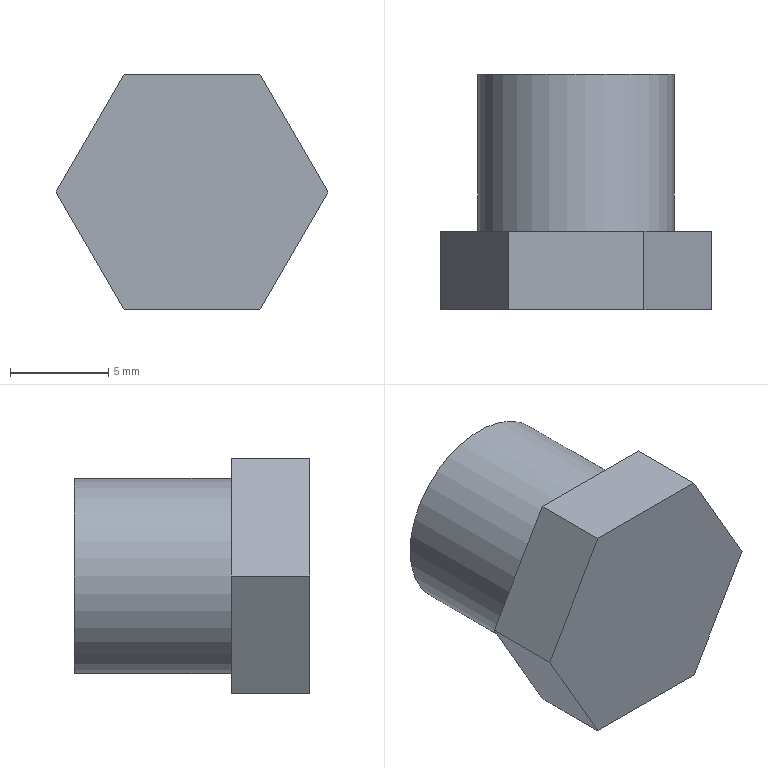Part | STEP file | 1-06.3 | 1 solid | 10 faces | box 13.856 x 12 x 12 mm | volume 1127 mm3 | plane 9 | cylinder 1 | commonest cylinder face diameters 10 x1
STEP:
#1=CARTESIAN_POINT('',(0.,0.,0.));
#2=DIRECTION('',(0.,0.,1.));
#3=DIRECTION('',(1.,0.,0.));
#4=AXIS2_PLACEMENT_3D('',#1,#2,#3);
#5=CARTESIAN_POINT('',(-6.928,-4.,0.));
#6=VERTEX_POINT('',#5);
#7=CARTESIAN_POINT('',(-3.464,-4.,6.));
#8=VERTEX_POINT('',#7);
#9=CARTESIAN_POINT('',(-6.928,-4.,0.));
#10=DIRECTION('',(0.5,0.,0.866));
#11=VECTOR('',#10,1.);
#12=LINE('',#9,#11);
#13=CARTESIAN_POINT('',(0.,-4.,-0.9282));
#14=DIRECTION('',(0.,1.,0.));
#15=DIRECTION('',(1.,0.,0.));
#16=AXIS2_PLACEMENT_3D('',#13,#14,#15);
#17=PLANE('',#16);
#18=CARTESIAN_POINT('',(-6.928,-0.9282));
#19=DIRECTION('',(0.5,-0.866));
#20=VECTOR('',#19,1.);
#21=LINE('',#18,#20);
#22=(GEOMETRIC_REPRESENTATION_CONTEXT(2)PARAMETRIC_REPRESENTATION_CONTEXT()REPRESENTATION_CONTEXT('',''));
#23=DEFINITIONAL_REPRESENTATION('',(#21),#22);
#24=PCURVE('',#17,#23);
#25=CARTESIAN_POINT('',(-5.196,-2.,3.));
#26=DIRECTION('',(0.866,0.,-0.5));
#27=DIRECTION('',(0.5,0.,0.866));
#28=AXIS2_PLACEMENT_3D('',#25,#26,#27);
#29=PLANE('',#28);
#30=CARTESIAN_POINT('',(-3.464,2.));
#31=DIRECTION('',(1.,0.));
#32=VECTOR('',#31,1.);
#33=LINE('',#30,#32);
#34=(GEOMETRIC_REPRESENTATION_CONTEXT(2)PARAMETRIC_REPRESENTATION_CONTEXT()REPRESENTATION_CONTEXT('',''));
#35=DEFINITIONAL_REPRESENTATION('',(#33),#34);
#36=PCURVE('',#29,#35);
#37=SURFACE_CURVE('',#12,(#24,#36),.PCURVE_S1.);
#38=EDGE_CURVE('',#6,#8,#37,.T.);
#39=ORIENTED_EDGE('',*,*,#38,.T.);
#40=CARTESIAN_POINT('',(3.464,-4.,6.));
#41=VERTEX_POINT('',#40);
#42=CARTESIAN_POINT('',(-3.464,-4.,6.));
#43=DIRECTION('',(1.,0.,0.));
#44=VECTOR('',#43,1.);
#45=LINE('',#42,#44);
#46=CARTESIAN_POINT('',(-3.464,-6.928));
#47=DIRECTION('',(1.,0.));
#48=VECTOR('',#47,1.);
#49=LINE('',#46,#48);
#50=(GEOMETRIC_REPRESENTATION_CONTEXT(2)PARAMETRIC_REPRESENTATION_CONTEXT()REPRESENTATION_CONTEXT('',''));
#51=DEFINITIONAL_REPRESENTATION('',(#49),#50);
#52=PCURVE('',#17,#51);
#53=CARTESIAN_POINT('',(0.,-2.,6.));
#54=DIRECTION('',(0.,0.,-1.));
#55=DIRECTION('',(1.,0.,0.));
#56=AXIS2_PLACEMENT_3D('',#53,#54,#55);
#57=PLANE('',#56);
#58=CARTESIAN_POINT('',(-3.464,2.));
#59=DIRECTION('',(1.,0.));
#60=VECTOR('',#59,1.);
#61=LINE('',#58,#60);
#62=(GEOMETRIC_REPRESENTATION_CONTEXT(2)PARAMETRIC_REPRESENTATION_CONTEXT()REPRESENTATION_CONTEXT('',''));
#63=DEFINITIONAL_REPRESENTATION('',(#61),#62);
#64=PCURVE('',#57,#63);
#65=SURFACE_CURVE('',#45,(#52,#64),.PCURVE_S1.);
#66=EDGE_CURVE('',#8,#41,#65,.T.);
#67=ORIENTED_EDGE('',*,*,#66,.T.);
#68=CARTESIAN_POINT('',(6.928,-4.,0.));
#69=VERTEX_POINT('',#68);
#70=CARTESIAN_POINT('',(3.464,-4.,6.));
#71=DIRECTION('',(0.5,0.,-0.866));
#72=VECTOR('',#71,1.);
#73=LINE('',#70,#72);
#74=CARTESIAN_POINT('',(3.464,-6.928));
#75=DIRECTION('',(0.5,0.866));
#76=VECTOR('',#75,1.);
#77=LINE('',#74,#76);
#78=(GEOMETRIC_REPRESENTATION_CONTEXT(2)PARAMETRIC_REPRESENTATION_CONTEXT()REPRESENTATION_CONTEXT('',''));
#79=DEFINITIONAL_REPRESENTATION('',(#77),#78);
#80=PCURVE('',#17,#79);
#81=CARTESIAN_POINT('',(5.196,-2.,3.));
#82=DIRECTION('',(-0.866,0.,-0.5));
#83=DIRECTION('',(0.5,0.,-0.866));
#84=AXIS2_PLACEMENT_3D('',#81,#82,#83);
#85=PLANE('',#84);
#86=CARTESIAN_POINT('',(-3.464,2.));
#87=DIRECTION('',(1.,0.));
#88=VECTOR('',#87,1.);
#89=LINE('',#86,#88);
#90=(GEOMETRIC_REPRESENTATION_CONTEXT(2)PARAMETRIC_REPRESENTATION_CONTEXT()REPRESENTATION_CONTEXT('',''));
#91=DEFINITIONAL_REPRESENTATION('',(#89),#90);
#92=PCURVE('',#85,#91);
#93=SURFACE_CURVE('',#73,(#80,#92),.PCURVE_S1.);
#94=EDGE_CURVE('',#41,#69,#93,.T.);
#95=ORIENTED_EDGE('',*,*,#94,.T.);
#96=CARTESIAN_POINT('',(3.464,-4.,-6.));
#97=VERTEX_POINT('',#96);
#98=CARTESIAN_POINT('',(6.928,-4.,0.));
#99=DIRECTION('',(-0.5,0.,-0.866));
#100=VECTOR('',#99,1.);
#101=LINE('',#98,#100);
#102=CARTESIAN_POINT('',(6.928,-0.9282));
#103=DIRECTION('',(-0.5,0.866));
#104=VECTOR('',#103,1.);
#105=LINE('',#102,#104);
#106=(GEOMETRIC_REPRESENTATION_CONTEXT(2)PARAMETRIC_REPRESENTATION_CONTEXT()REPRESENTATION_CONTEXT('',''));
#107=DEFINITIONAL_REPRESENTATION('',(#105),#106);
#108=PCURVE('',#17,#107);
#109=CARTESIAN_POINT('',(5.196,-2.,-3.));
#110=DIRECTION('',(-0.866,0.,0.5));
#111=DIRECTION('',(-0.5,0.,-0.866));
#112=AXIS2_PLACEMENT_3D('',#109,#110,#111);
#113=PLANE('',#112);
#114=CARTESIAN_POINT('',(-3.464,2.));
#115=DIRECTION('',(1.,0.));
#116=VECTOR('',#115,1.);
#117=LINE('',#114,#116);
#118=(GEOMETRIC_REPRESENTATION_CONTEXT(2)PARAMETRIC_REPRESENTATION_CONTEXT()REPRESENTATION_CONTEXT('',''));
#119=DEFINITIONAL_REPRESENTATION('',(#117),#118);
#120=PCURVE('',#113,#119);
#121=SURFACE_CURVE('',#101,(#108,#120),.PCURVE_S1.);
#122=EDGE_CURVE('',#69,#97,#121,.T.);
#123=ORIENTED_EDGE('',*,*,#122,.T.);
#124=CARTESIAN_POINT('',(-3.464,-4.,-6.));
#125=VERTEX_POINT('',#124);
#126=CARTESIAN_POINT('',(3.464,-4.,-6.));
#127=DIRECTION('',(-1.,0.,0.));
#128=VECTOR('',#127,1.);
#129=LINE('',#126,#128);
#130=CARTESIAN_POINT('',(3.464,5.072));
#131=DIRECTION('',(-1.,0.));
#132=VECTOR('',#131,1.);
#133=LINE('',#130,#132);
#134=(GEOMETRIC_REPRESENTATION_CONTEXT(2)PARAMETRIC_REPRESENTATION_CONTEXT()REPRESENTATION_CONTEXT('',''));
#135=DEFINITIONAL_REPRESENTATION('',(#133),#134);
#136=PCURVE('',#17,#135);
#137=CARTESIAN_POINT('',(0.,-2.,-6.));
#138=DIRECTION('',(0.,0.,1.));
#139=DIRECTION('',(-1.,0.,0.));
#140=AXIS2_PLACEMENT_3D('',#137,#138,#139);
#141=PLANE('',#140);
#142=CARTESIAN_POINT('',(-3.464,2.));
#143=DIRECTION('',(1.,0.));
#144=VECTOR('',#143,1.);
#145=LINE('',#142,#144);
#146=(GEOMETRIC_REPRESENTATION_CONTEXT(2)PARAMETRIC_REPRESENTATION_CONTEXT()REPRESENTATION_CONTEXT('',''));
#147=DEFINITIONAL_REPRESENTATION('',(#145),#146);
#148=PCURVE('',#141,#147);
#149=SURFACE_CURVE('',#129,(#136,#148),.PCURVE_S1.);
#150=EDGE_CURVE('',#97,#125,#149,.T.);
#151=ORIENTED_EDGE('',*,*,#150,.T.);
#152=CARTESIAN_POINT('',(-3.464,-4.,-6.));
#153=DIRECTION('',(-0.5,0.,0.866));
#154=VECTOR('',#153,1.);
#155=LINE('',#152,#154);
#156=CARTESIAN_POINT('',(-3.464,5.072));
#157=DIRECTION('',(-0.5,-0.866));
#158=VECTOR('',#157,1.);
#159=LINE('',#156,#158);
#160=(GEOMETRIC_REPRESENTATION_CONTEXT(2)PARAMETRIC_REPRESENTATION_CONTEXT()REPRESENTATION_CONTEXT('',''));
#161=DEFINITIONAL_REPRESENTATION('',(#159),#160);
#162=PCURVE('',#17,#161);
#163=CARTESIAN_POINT('',(-5.196,-2.,-3.));
#164=DIRECTION('',(0.866,0.,0.5));
#165=DIRECTION('',(-0.5,0.,0.866));
#166=AXIS2_PLACEMENT_3D('',#163,#164,#165);
#167=PLANE('',#166);
#168=CARTESIAN_POINT('',(-3.464,2.));
#169=DIRECTION('',(1.,0.));
#170=VECTOR('',#169,1.);
#171=LINE('',#168,#170);
#172=(GEOMETRIC_REPRESENTATION_CONTEXT(2)PARAMETRIC_REPRESENTATION_CONTEXT()REPRESENTATION_CONTEXT('',''));
#173=DEFINITIONAL_REPRESENTATION('',(#171),#172);
#174=PCURVE('',#167,#173);
#175=SURFACE_CURVE('',#155,(#162,#174),.PCURVE_S1.);
#176=EDGE_CURVE('',#125,#6,#175,.T.);
#177=ORIENTED_EDGE('',*,*,#176,.T.);
#178=EDGE_LOOP('',(#39,#67,#95,#123,#151,#177));
#179=FACE_BOUND('',#178,.F.);
#180=ADVANCED_FACE('',(#179),#17,.F.);
#181=CARTESIAN_POINT('',(-6.928,0.,0.));
#182=VERTEX_POINT('',#181);
#183=CARTESIAN_POINT('',(-3.464,0.,6.));
#184=VERTEX_POINT('',#183);
#185=CARTESIAN_POINT('',(-6.928,0.,0.));
#186=DIRECTION('',(0.5,0.,0.866));
#187=VECTOR('',#186,1.);
#188=LINE('',#185,#187);
#189=CARTESIAN_POINT('',(-3.464,-2.));
#190=DIRECTION('',(1.,0.));
#191=VECTOR('',#190,1.);
#192=LINE('',#189,#191);
#193=(GEOMETRIC_REPRESENTATION_CONTEXT(2)PARAMETRIC_REPRESENTATION_CONTEXT()REPRESENTATION_CONTEXT('',''));
#194=DEFINITIONAL_REPRESENTATION('',(#192),#193);
#195=PCURVE('',#29,#194);
#196=CARTESIAN_POINT('',(0.,0.,-0.9282));
#197=DIRECTION('',(0.,1.,0.));
#198=DIRECTION('',(1.,0.,0.));
#199=AXIS2_PLACEMENT_3D('',#196,#197,#198);
#200=PLANE('',#199);
#201=CARTESIAN_POINT('',(-6.928,-0.9282));
#202=DIRECTION('',(0.5,-0.866));
#203=VECTOR('',#202,1.);
#204=LINE('',#201,#203);
#205=(GEOMETRIC_REPRESENTATION_CONTEXT(2)PARAMETRIC_REPRESENTATION_CONTEXT()REPRESENTATION_CONTEXT('',''));
#206=DEFINITIONAL_REPRESENTATION('',(#204),#205);
#207=PCURVE('',#200,#206);
#208=SURFACE_CURVE('',#188,(#195,#207),.PCURVE_S1.);
#209=EDGE_CURVE('',#182,#184,#208,.T.);
#210=ORIENTED_EDGE('',*,*,#209,.T.);
#211=CARTESIAN_POINT('',(-3.464,0.,6.));
#212=DIRECTION('',(0.,-1.,0.));
#213=VECTOR('',#212,1.);
#214=LINE('',#211,#213);
#215=CARTESIAN_POINT('',(3.464,-2.));
#216=DIRECTION('',(0.,1.));
#217=VECTOR('',#216,1.);
#218=LINE('',#215,#217);
#219=(GEOMETRIC_REPRESENTATION_CONTEXT(2)PARAMETRIC_REPRESENTATION_CONTEXT()REPRESENTATION_CONTEXT('',''));
#220=DEFINITIONAL_REPRESENTATION('',(#218),#219);
#221=PCURVE('',#29,#220);
#222=CARTESIAN_POINT('',(-3.464,-2.));
#223=DIRECTION('',(0.,1.));
#224=VECTOR('',#223,1.);
#225=LINE('',#222,#224);
#226=(GEOMETRIC_REPRESENTATION_CONTEXT(2)PARAMETRIC_REPRESENTATION_CONTEXT()REPRESENTATION_CONTEXT('',''));
#227=DEFINITIONAL_REPRESENTATION('',(#225),#226);
#228=PCURVE('',#57,#227);
#229=SURFACE_CURVE('',#214,(#221,#228),.PCURVE_S1.);
#230=EDGE_CURVE('',#184,#8,#229,.T.);
#231=ORIENTED_EDGE('',*,*,#230,.T.);
#232=ORIENTED_EDGE('',*,*,#38,.F.);
#233=CARTESIAN_POINT('',(-6.928,0.,0.));
#234=DIRECTION('',(0.,-1.,0.));
#235=VECTOR('',#234,1.);
#236=LINE('',#233,#235);
#237=CARTESIAN_POINT('',(-3.464,-2.));
#238=DIRECTION('',(0.,1.));
#239=VECTOR('',#238,1.);
#240=LINE('',#237,#239);
#241=(GEOMETRIC_REPRESENTATION_CONTEXT(2)PARAMETRIC_REPRESENTATION_CONTEXT()REPRESENTATION_CONTEXT('',''));
#242=DEFINITIONAL_REPRESENTATION('',(#240),#241);
#243=PCURVE('',#29,#242);
#244=CARTESIAN_POINT('',(3.464,-2.));
#245=DIRECTION('',(0.,1.));
#246=VECTOR('',#245,1.);
#247=LINE('',#244,#246);
#248=(GEOMETRIC_REPRESENTATION_CONTEXT(2)PARAMETRIC_REPRESENTATION_CONTEXT()REPRESENTATION_CONTEXT('',''));
#249=DEFINITIONAL_REPRESENTATION('',(#247),#248);
#250=PCURVE('',#167,#249);
#251=SURFACE_CURVE('',#236,(#243,#250),.PCURVE_S1.);
#252=EDGE_CURVE('',#182,#6,#251,.T.);
#253=ORIENTED_EDGE('',*,*,#252,.F.);
#254=EDGE_LOOP('',(#210,#231,#232,#253));
#255=FACE_BOUND('',#254,.F.);
#256=ADVANCED_FACE('',(#255),#29,.F.);
#257=CARTESIAN_POINT('',(3.464,0.,6.));
#258=VERTEX_POINT('',#257);
#259=CARTESIAN_POINT('',(-3.464,0.,6.));
#260=DIRECTION('',(1.,0.,0.));
#261=VECTOR('',#260,1.);
#262=LINE('',#259,#261);
#263=CARTESIAN_POINT('',(-3.464,-2.));
#264=DIRECTION('',(1.,0.));
#265=VECTOR('',#264,1.);
#266=LINE('',#263,#265);
#267=(GEOMETRIC_REPRESENTATION_CONTEXT(2)PARAMETRIC_REPRESENTATION_CONTEXT()REPRESENTATION_CONTEXT('',''));
#268=DEFINITIONAL_REPRESENTATION('',(#266),#267);
#269=PCURVE('',#57,#268);
#270=CARTESIAN_POINT('',(-3.464,-6.928));
#271=DIRECTION('',(1.,0.));
#272=VECTOR('',#271,1.);
#273=LINE('',#270,#272);
#274=(GEOMETRIC_REPRESENTATION_CONTEXT(2)PARAMETRIC_REPRESENTATION_CONTEXT()REPRESENTATION_CONTEXT('',''));
#275=DEFINITIONAL_REPRESENTATION('',(#273),#274);
#276=PCURVE('',#200,#275);
#277=SURFACE_CURVE('',#262,(#269,#276),.PCURVE_S1.);
#278=EDGE_CURVE('',#184,#258,#277,.T.);
#279=ORIENTED_EDGE('',*,*,#278,.T.);
#280=CARTESIAN_POINT('',(3.464,0.,6.));
#281=DIRECTION('',(0.,-1.,0.));
#282=VECTOR('',#281,1.);
#283=LINE('',#280,#282);
#284=CARTESIAN_POINT('',(3.464,-2.));
#285=DIRECTION('',(0.,1.));
#286=VECTOR('',#285,1.);
#287=LINE('',#284,#286);
#288=(GEOMETRIC_REPRESENTATION_CONTEXT(2)PARAMETRIC_REPRESENTATION_CONTEXT()REPRESENTATION_CONTEXT('',''));
#289=DEFINITIONAL_REPRESENTATION('',(#287),#288);
#290=PCURVE('',#57,#289);
#291=CARTESIAN_POINT('',(-3.464,-2.));
#292=DIRECTION('',(0.,1.));
#293=VECTOR('',#292,1.);
#294=LINE('',#291,#293);
#295=(GEOMETRIC_REPRESENTATION_CONTEXT(2)PARAMETRIC_REPRESENTATION_CONTEXT()REPRESENTATION_CONTEXT('',''));
#296=DEFINITIONAL_REPRESENTATION('',(#294),#295);
#297=PCURVE('',#85,#296);
#298=SURFACE_CURVE('',#283,(#290,#297),.PCURVE_S1.);
#299=EDGE_CURVE('',#258,#41,#298,.T.);
#300=ORIENTED_EDGE('',*,*,#299,.T.);
#301=ORIENTED_EDGE('',*,*,#66,.F.);
#302=ORIENTED_EDGE('',*,*,#230,.F.);
#303=EDGE_LOOP('',(#279,#300,#301,#302));
#304=FACE_BOUND('',#303,.F.);
#305=ADVANCED_FACE('',(#304),#57,.F.);
#306=CARTESIAN_POINT('',(6.928,0.,0.));
#307=VERTEX_POINT('',#306);
#308=CARTESIAN_POINT('',(3.464,0.,6.));
#309=DIRECTION('',(0.5,0.,-0.866));
#310=VECTOR('',#309,1.);
#311=LINE('',#308,#310);
#312=CARTESIAN_POINT('',(-3.464,-2.));
#313=DIRECTION('',(1.,0.));
#314=VECTOR('',#313,1.);
#315=LINE('',#312,#314);
#316=(GEOMETRIC_REPRESENTATION_CONTEXT(2)PARAMETRIC_REPRESENTATION_CONTEXT()REPRESENTATION_CONTEXT('',''));
#317=DEFINITIONAL_REPRESENTATION('',(#315),#316);
#318=PCURVE('',#85,#317);
#319=CARTESIAN_POINT('',(3.464,-6.928));
#320=DIRECTION('',(0.5,0.866));
#321=VECTOR('',#320,1.);
#322=LINE('',#319,#321);
#323=(GEOMETRIC_REPRESENTATION_CONTEXT(2)PARAMETRIC_REPRESENTATION_CONTEXT()REPRESENTATION_CONTEXT('',''));
#324=DEFINITIONAL_REPRESENTATION('',(#322),#323);
#325=PCURVE('',#200,#324);
#326=SURFACE_CURVE('',#311,(#318,#325),.PCURVE_S1.);
#327=EDGE_CURVE('',#258,#307,#326,.T.);
#328=ORIENTED_EDGE('',*,*,#327,.T.);
#329=CARTESIAN_POINT('',(6.928,0.,0.));
#330=DIRECTION('',(0.,-1.,0.));
#331=VECTOR('',#330,1.);
#332=LINE('',#329,#331);
#333=CARTESIAN_POINT('',(3.464,-2.));
#334=DIRECTION('',(0.,1.));
#335=VECTOR('',#334,1.);
#336=LINE('',#333,#335);
#337=(GEOMETRIC_REPRESENTATION_CONTEXT(2)PARAMETRIC_REPRESENTATION_CONTEXT()REPRESENTATION_CONTEXT('',''));
#338=DEFINITIONAL_REPRESENTATION('',(#336),#337);
#339=PCURVE('',#85,#338);
#340=CARTESIAN_POINT('',(-3.464,-2.));
#341=DIRECTION('',(0.,1.));
#342=VECTOR('',#341,1.);
#343=LINE('',#340,#342);
#344=(GEOMETRIC_REPRESENTATION_CONTEXT(2)PARAMETRIC_REPRESENTATION_CONTEXT()REPRESENTATION_CONTEXT('',''));
#345=DEFINITIONAL_REPRESENTATION('',(#343),#344);
#346=PCURVE('',#113,#345);
#347=SURFACE_CURVE('',#332,(#339,#346),.PCURVE_S1.);
#348=EDGE_CURVE('',#307,#69,#347,.T.);
#349=ORIENTED_EDGE('',*,*,#348,.T.);
#350=ORIENTED_EDGE('',*,*,#94,.F.);
#351=ORIENTED_EDGE('',*,*,#299,.F.);
#352=EDGE_LOOP('',(#328,#349,#350,#351));
#353=FACE_BOUND('',#352,.F.);
#354=ADVANCED_FACE('',(#353),#85,.F.);
#355=CARTESIAN_POINT('',(3.464,0.,-6.));
#356=VERTEX_POINT('',#355);
#357=CARTESIAN_POINT('',(6.928,0.,0.));
#358=DIRECTION('',(-0.5,0.,-0.866));
#359=VECTOR('',#358,1.);
#360=LINE('',#357,#359);
#361=CARTESIAN_POINT('',(-3.464,-2.));
#362=DIRECTION('',(1.,0.));
#363=VECTOR('',#362,1.);
#364=LINE('',#361,#363);
#365=(GEOMETRIC_REPRESENTATION_CONTEXT(2)PARAMETRIC_REPRESENTATION_CONTEXT()REPRESENTATION_CONTEXT('',''));
#366=DEFINITIONAL_REPRESENTATION('',(#364),#365);
#367=PCURVE('',#113,#366);
#368=CARTESIAN_POINT('',(6.928,-0.9282));
#369=DIRECTION('',(-0.5,0.866));
#370=VECTOR('',#369,1.);
#371=LINE('',#368,#370);
#372=(GEOMETRIC_REPRESENTATION_CONTEXT(2)PARAMETRIC_REPRESENTATION_CONTEXT()REPRESENTATION_CONTEXT('',''));
#373=DEFINITIONAL_REPRESENTATION('',(#371),#372);
#374=PCURVE('',#200,#373);
#375=SURFACE_CURVE('',#360,(#367,#374),.PCURVE_S1.);
#376=EDGE_CURVE('',#307,#356,#375,.T.);
#377=ORIENTED_EDGE('',*,*,#376,.T.);
#378=CARTESIAN_POINT('',(3.464,0.,-6.));
#379=DIRECTION('',(0.,-1.,0.));
#380=VECTOR('',#379,1.);
#381=LINE('',#378,#380);
#382=CARTESIAN_POINT('',(3.464,-2.));
#383=DIRECTION('',(0.,1.));
#384=VECTOR('',#383,1.);
#385=LINE('',#382,#384);
#386=(GEOMETRIC_REPRESENTATION_CONTEXT(2)PARAMETRIC_REPRESENTATION_CONTEXT()REPRESENTATION_CONTEXT('',''));
#387=DEFINITIONAL_REPRESENTATION('',(#385),#386);
#388=PCURVE('',#113,#387);
#389=CARTESIAN_POINT('',(-3.464,-2.));
#390=DIRECTION('',(0.,1.));
#391=VECTOR('',#390,1.);
#392=LINE('',#389,#391);
#393=(GEOMETRIC_REPRESENTATION_CONTEXT(2)PARAMETRIC_REPRESENTATION_CONTEXT()REPRESENTATION_CONTEXT('',''));
#394=DEFINITIONAL_REPRESENTATION('',(#392),#393);
#395=PCURVE('',#141,#394);
#396=SURFACE_CURVE('',#381,(#388,#395),.PCURVE_S1.);
#397=EDGE_CURVE('',#356,#97,#396,.T.);
#398=ORIENTED_EDGE('',*,*,#397,.T.);
#399=ORIENTED_EDGE('',*,*,#122,.F.);
#400=ORIENTED_EDGE('',*,*,#348,.F.);
#401=EDGE_LOOP('',(#377,#398,#399,#400));
#402=FACE_BOUND('',#401,.F.);
#403=ADVANCED_FACE('',(#402),#113,.F.);
#404=CARTESIAN_POINT('',(-3.464,0.,-6.));
#405=VERTEX_POINT('',#404);
#406=CARTESIAN_POINT('',(3.464,0.,-6.));
#407=DIRECTION('',(-1.,0.,0.));
#408=VECTOR('',#407,1.);
#409=LINE('',#406,#408);
#410=CARTESIAN_POINT('',(-3.464,-2.));
#411=DIRECTION('',(1.,0.));
#412=VECTOR('',#411,1.);
#413=LINE('',#410,#412);
#414=(GEOMETRIC_REPRESENTATION_CONTEXT(2)PARAMETRIC_REPRESENTATION_CONTEXT()REPRESENTATION_CONTEXT('',''));
#415=DEFINITIONAL_REPRESENTATION('',(#413),#414);
#416=PCURVE('',#141,#415);
#417=CARTESIAN_POINT('',(3.464,5.072));
#418=DIRECTION('',(-1.,0.));
#419=VECTOR('',#418,1.);
#420=LINE('',#417,#419);
#421=(GEOMETRIC_REPRESENTATION_CONTEXT(2)PARAMETRIC_REPRESENTATION_CONTEXT()REPRESENTATION_CONTEXT('',''));
#422=DEFINITIONAL_REPRESENTATION('',(#420),#421);
#423=PCURVE('',#200,#422);
#424=SURFACE_CURVE('',#409,(#416,#423),.PCURVE_S1.);
#425=EDGE_CURVE('',#356,#405,#424,.T.);
#426=ORIENTED_EDGE('',*,*,#425,.T.);
#427=CARTESIAN_POINT('',(-3.464,0.,-6.));
#428=DIRECTION('',(0.,-1.,0.));
#429=VECTOR('',#428,1.);
#430=LINE('',#427,#429);
#431=CARTESIAN_POINT('',(3.464,-2.));
#432=DIRECTION('',(0.,1.));
#433=VECTOR('',#432,1.);
#434=LINE('',#431,#433);
#435=(GEOMETRIC_REPRESENTATION_CONTEXT(2)PARAMETRIC_REPRESENTATION_CONTEXT()REPRESENTATION_CONTEXT('',''));
#436=DEFINITIONAL_REPRESENTATION('',(#434),#435);
#437=PCURVE('',#141,#436);
#438=CARTESIAN_POINT('',(-3.464,-2.));
#439=DIRECTION('',(0.,1.));
#440=VECTOR('',#439,1.);
#441=LINE('',#438,#440);
#442=(GEOMETRIC_REPRESENTATION_CONTEXT(2)PARAMETRIC_REPRESENTATION_CONTEXT()REPRESENTATION_CONTEXT('',''));
#443=DEFINITIONAL_REPRESENTATION('',(#441),#442);
#444=PCURVE('',#167,#443);
#445=SURFACE_CURVE('',#430,(#437,#444),.PCURVE_S1.);
#446=EDGE_CURVE('',#405,#125,#445,.T.);
#447=ORIENTED_EDGE('',*,*,#446,.T.);
#448=ORIENTED_EDGE('',*,*,#150,.F.);
#449=ORIENTED_EDGE('',*,*,#397,.F.);
#450=EDGE_LOOP('',(#426,#447,#448,#449));
#451=FACE_BOUND('',#450,.F.);
#452=ADVANCED_FACE('',(#451),#141,.F.);
#453=CARTESIAN_POINT('',(-3.464,0.,-6.));
#454=DIRECTION('',(-0.5,0.,0.866));
#455=VECTOR('',#454,1.);
#456=LINE('',#453,#455);
#457=CARTESIAN_POINT('',(-3.464,-2.));
#458=DIRECTION('',(1.,0.));
#459=VECTOR('',#458,1.);
#460=LINE('',#457,#459);
#461=(GEOMETRIC_REPRESENTATION_CONTEXT(2)PARAMETRIC_REPRESENTATION_CONTEXT()REPRESENTATION_CONTEXT('',''));
#462=DEFINITIONAL_REPRESENTATION('',(#460),#461);
#463=PCURVE('',#167,#462);
#464=CARTESIAN_POINT('',(-3.464,5.072));
#465=DIRECTION('',(-0.5,-0.866));
#466=VECTOR('',#465,1.);
#467=LINE('',#464,#466);
#468=(GEOMETRIC_REPRESENTATION_CONTEXT(2)PARAMETRIC_REPRESENTATION_CONTEXT()REPRESENTATION_CONTEXT('',''));
#469=DEFINITIONAL_REPRESENTATION('',(#467),#468);
#470=PCURVE('',#200,#469);
#471=SURFACE_CURVE('',#456,(#463,#470),.PCURVE_S1.);
#472=EDGE_CURVE('',#405,#182,#471,.T.);
#473=ORIENTED_EDGE('',*,*,#472,.T.);
#474=ORIENTED_EDGE('',*,*,#252,.T.);
#475=ORIENTED_EDGE('',*,*,#176,.F.);
#476=ORIENTED_EDGE('',*,*,#446,.F.);
#477=EDGE_LOOP('',(#473,#474,#475,#476));
#478=FACE_BOUND('',#477,.F.);
#479=ADVANCED_FACE('',(#478),#167,.F.);
#480=ORIENTED_EDGE('',*,*,#209,.T.);
#481=ORIENTED_EDGE('',*,*,#278,.T.);
#482=ORIENTED_EDGE('',*,*,#327,.T.);
#483=ORIENTED_EDGE('',*,*,#376,.T.);
#484=ORIENTED_EDGE('',*,*,#425,.T.);
#485=ORIENTED_EDGE('',*,*,#472,.T.);
#486=EDGE_LOOP('',(#480,#481,#482,#483,#484,#485));
#487=FACE_BOUND('',#486,.T.);
#488=CARTESIAN_POINT('',(5.,0.,0.));
#489=VERTEX_POINT('',#488);
#490=CARTESIAN_POINT('',(0.,0.,0.));
#491=DIRECTION('',(0.,-1.,0.));
#492=DIRECTION('',(1.,0.,0.));
#493=AXIS2_PLACEMENT_3D('',#490,#491,#492);
#494=CIRCLE('',#493,5.);
#495=CARTESIAN_POINT('',(5.,-0.9282));
#496=CARTESIAN_POINT('',(5.,-9.588));
#497=CARTESIAN_POINT('',(-2.5,-5.258));
#498=CARTESIAN_POINT('',(-10.,-0.9282));
#499=CARTESIAN_POINT('',(-2.5,3.402));
#500=CARTESIAN_POINT('',(5.,7.732));
#501=CARTESIAN_POINT('',(5.,-0.9282));
#502=(BOUNDED_CURVE()B_SPLINE_CURVE(2,(#495,#496,#497,#498,#499,#500,#501),.UNSPECIFIED.,.T.,.F.)B_SPLINE_CURVE_WITH_KNOTS((1,2,2,2,2,1),(-2.094,0.,2.094,4.189,6.283,8.378),.UNSPECIFIED.)CURVE()GEOMETRIC_REPRESENTATION_ITEM()RATIONAL_B_SPLINE_CURVE((1.,0.5,1.,0.5,1.,0.5,1.))REPRESENTATION_ITEM(''));
#503=(GEOMETRIC_REPRESENTATION_CONTEXT(2)PARAMETRIC_REPRESENTATION_CONTEXT()REPRESENTATION_CONTEXT('',''));
#504=DEFINITIONAL_REPRESENTATION('',(#502),#503);
#505=PCURVE('',#200,#504);
#506=CARTESIAN_POINT('',(0.,0.,0.));
#507=DIRECTION('',(0.,1.,0.));
#508=DIRECTION('',(1.,0.,0.));
#509=AXIS2_PLACEMENT_3D('',#506,#507,#508);
#510=CYLINDRICAL_SURFACE('',#509,5.);
#511=CARTESIAN_POINT('',(6.283,0.));
#512=DIRECTION('',(-1.,0.));
#513=VECTOR('',#512,1.);
#514=LINE('',#511,#513);
#515=(GEOMETRIC_REPRESENTATION_CONTEXT(2)PARAMETRIC_REPRESENTATION_CONTEXT()REPRESENTATION_CONTEXT('',''));
#516=DEFINITIONAL_REPRESENTATION('',(#514),#515);
#517=PCURVE('',#510,#516);
#518=SURFACE_CURVE('',#494,(#505,#517),.PCURVE_S1.);
#519=EDGE_CURVE('',#489,#489,#518,.T.);
#520=ORIENTED_EDGE('',*,*,#519,.T.);
#521=EDGE_LOOP('',(#520));
#522=FACE_BOUND('',#521,.T.);
#523=ADVANCED_FACE('',(#487,#522),#200,.T.);
#524=CARTESIAN_POINT('',(5.,8.,0.));
#525=VERTEX_POINT('',#524);
#526=CARTESIAN_POINT('',(5.,0.,0.));
#527=DIRECTION('',(0.,1.,0.));
#528=VECTOR('',#527,1.);
#529=LINE('',#526,#528);
#530=CARTESIAN_POINT('',(6.283,0.));
#531=DIRECTION('',(0.,1.));
#532=VECTOR('',#531,1.);
#533=LINE('',#530,#532);
#534=(GEOMETRIC_REPRESENTATION_CONTEXT(2)PARAMETRIC_REPRESENTATION_CONTEXT()REPRESENTATION_CONTEXT('',''));
#535=DEFINITIONAL_REPRESENTATION('',(#533),#534);
#536=PCURVE('',#510,#535);
#537=CARTESIAN_POINT('',(0.,0.));
#538=DIRECTION('',(0.,1.));
#539=VECTOR('',#538,1.);
#540=LINE('',#537,#539);
#541=(GEOMETRIC_REPRESENTATION_CONTEXT(2)PARAMETRIC_REPRESENTATION_CONTEXT()REPRESENTATION_CONTEXT('',''));
#542=DEFINITIONAL_REPRESENTATION('',(#540),#541);
#543=PCURVE('',#510,#542);
#544=SEAM_CURVE('',#529,(#536,#543),.PCURVE_S1.);
#545=EDGE_CURVE('',#489,#525,#544,.T.);
#546=ORIENTED_EDGE('',*,*,#545,.T.);
#547=CARTESIAN_POINT('',(0.,8.,0.));
#548=DIRECTION('',(0.,-1.,0.));
#549=DIRECTION('',(1.,0.,0.));
#550=AXIS2_PLACEMENT_3D('',#547,#548,#549);
#551=CIRCLE('',#550,5.);
#552=CARTESIAN_POINT('',(6.283,8.));
#553=DIRECTION('',(-1.,0.));
#554=VECTOR('',#553,1.);
#555=LINE('',#552,#554);
#556=(GEOMETRIC_REPRESENTATION_CONTEXT(2)PARAMETRIC_REPRESENTATION_CONTEXT()REPRESENTATION_CONTEXT('',''));
#557=DEFINITIONAL_REPRESENTATION('',(#555),#556);
#558=PCURVE('',#510,#557);
#559=CARTESIAN_POINT('',(-1.34,8.,0.));
#560=DIRECTION('',(0.,-1.,0.));
#561=DIRECTION('',(1.,0.,0.));
#562=AXIS2_PLACEMENT_3D('',#559,#560,#561);
#563=PLANE('',#562);
#564=CARTESIAN_POINT('',(1.34,0.));
#565=DIRECTION('',(1.,0.));
#566=AXIS2_PLACEMENT_2D('',#564,#565);
#567=CIRCLE('',#566,5.);
#568=(GEOMETRIC_REPRESENTATION_CONTEXT(2)PARAMETRIC_REPRESENTATION_CONTEXT()REPRESENTATION_CONTEXT('',''));
#569=DEFINITIONAL_REPRESENTATION('',(#567),#568);
#570=PCURVE('',#563,#569);
#571=SURFACE_CURVE('',#551,(#558,#570),.PCURVE_S1.);
#572=EDGE_CURVE('',#525,#525,#571,.T.);
#573=ORIENTED_EDGE('',*,*,#572,.T.);
#574=ORIENTED_EDGE('',*,*,#545,.F.);
#575=ORIENTED_EDGE('',*,*,#519,.F.);
#576=EDGE_LOOP('',(#546,#573,#574,#575));
#577=FACE_BOUND('',#576,.T.);
#578=ADVANCED_FACE('',(#577),#510,.T.);
#579=ORIENTED_EDGE('',*,*,#572,.T.);
#580=EDGE_LOOP('',(#579));
#581=FACE_BOUND('',#580,.F.);
#582=ADVANCED_FACE('',(#581),#563,.F.);
#583=CLOSED_SHELL('',(#180,#256,#305,#354,#403,#452,#479,#523,#578,#582));
#584=MANIFOLD_SOLID_BREP('',#583);
#585=(LENGTH_UNIT()NAMED_UNIT(*)SI_UNIT(.MILLI.,.METRE.));
#586=UNCERTAINTY_MEASURE_WITH_UNIT(LENGTH_MEASURE(0.0000001),#585,'','');
#587=(NAMED_UNIT(*)PLANE_ANGLE_UNIT()SI_UNIT($,.RADIAN.));
#588=(NAMED_UNIT(*)SI_UNIT($,.STERADIAN.)SOLID_ANGLE_UNIT());
#589=(GEOMETRIC_REPRESENTATION_CONTEXT(3)GLOBAL_UNCERTAINTY_ASSIGNED_CONTEXT((#586))GLOBAL_UNIT_ASSIGNED_CONTEXT((#585,#587,#588))REPRESENTATION_CONTEXT('',''));
#590=ADVANCED_BREP_SHAPE_REPRESENTATION('',(#4,#584),#589);